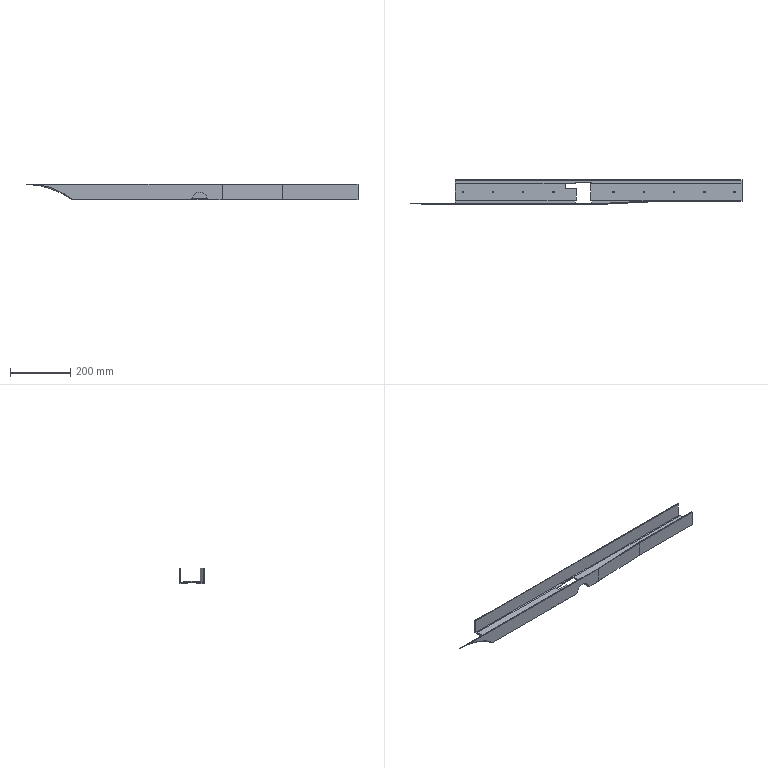Part | SolidWorks | features BaseBody 1 | 1 solid | 58 faces | box 1100 x 80 x 50 mm | volume 539674 mm3 | plane 38 | cylinder 19 | torus 1 | commonest cylinder face diameters 5 x18 50 x1